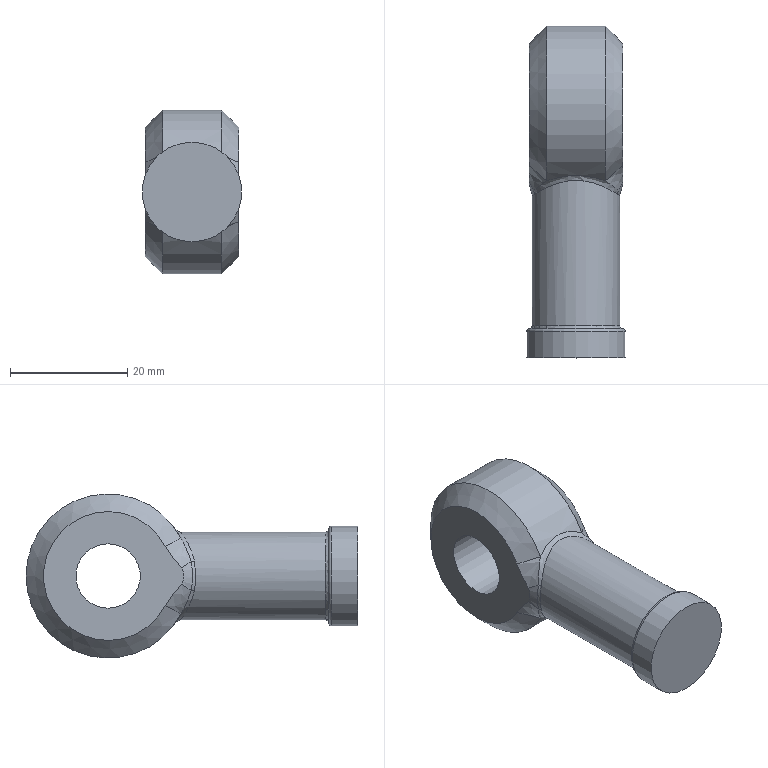Part | STEP file | Tube necking machine_id630_x_t | 1 solid | 21 faces | box 17 x 56.65 x 28 mm | volume 13077 mm3 | spline 10 | cylinder 4 | plane 3 | torus 2 | cone 2 | commonest cylinder face diameters 11 x1 15 x1 17 x1 28 x1